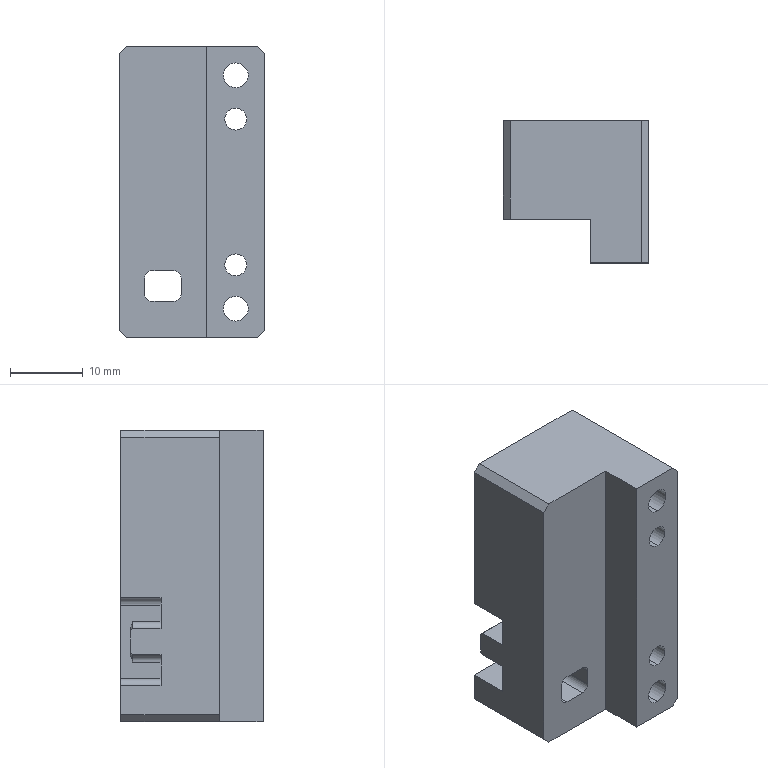Part | STEP file | PN_0022 | 1 solid | 53 faces | box 20 x 19.5 x 40 mm | volume 11103 mm3 | plane 27 | cylinder 24 | cone 2 | commonest cylinder face diameters 2 x8 3 x4 3.4 x4 6 x4 2.5 x2 3.2 x2